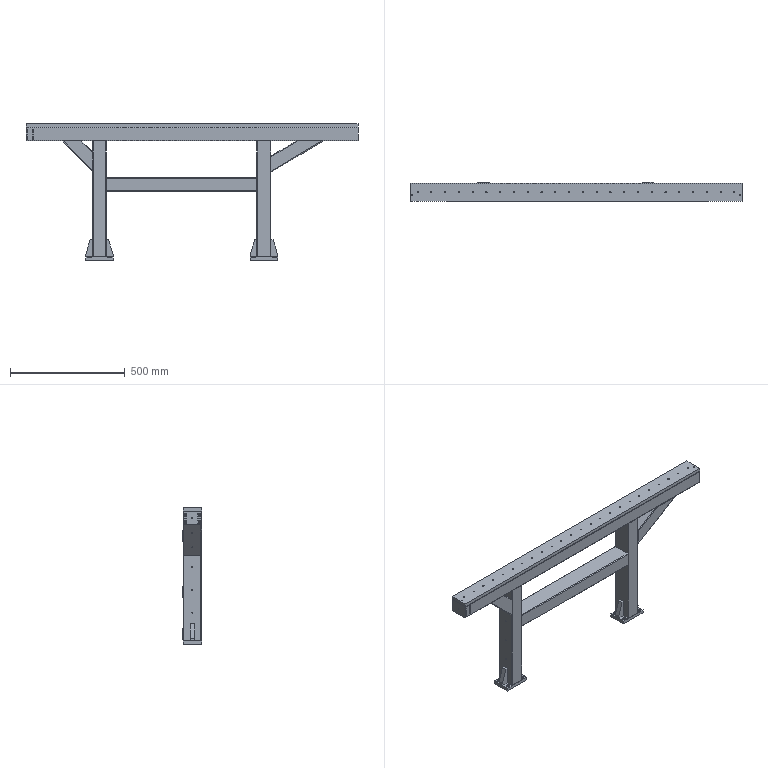Part | NX | 18 solids | 355 faces | box 1446 x 83.017 x 595 mm | volume 7511114 mm3 | plane 182 | cylinder 159 | cone 14 | commonest cylinder face diameters 5 x50 5.236 x48 4.2 x23 3.3 x20 9 x8 18 x8